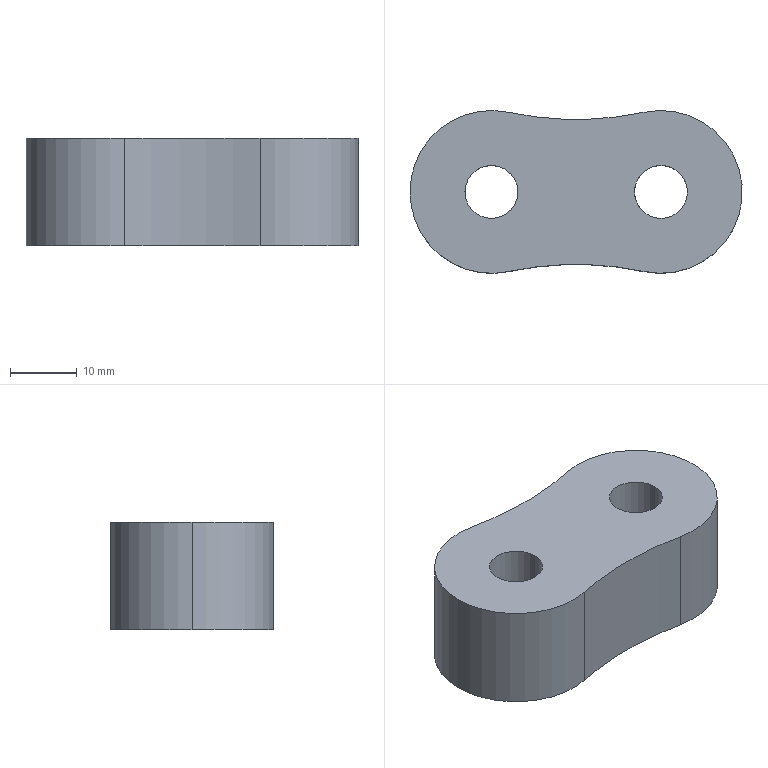Part | STEP file | Outer chain link pad block | 1 solid | 14 faces | box 49.79 x 24.39 x 16.175 mm | volume 15316 mm3 | cylinder 9 | plane 5 | commonest cylinder face diameters 7.94 x4 24.39 x3 97.627 x2
STEP:
#1=CARTESIAN_POINT('',(0.,0.,0.));
#2=DIRECTION('',(0.,0.,1.));
#3=DIRECTION('',(1.,0.,0.));
#4=AXIS2_PLACEMENT_3D('',#1,#2,#3);
#5=CARTESIAN_POINT('',(8.73,-0.05,-12.745));
#6=VERTEX_POINT('',#5);
#7=CARTESIAN_POINT('',(8.73,-0.05,-12.645));
#8=VERTEX_POINT('',#7);
#9=CARTESIAN_POINT('',(8.73,-0.05,0.));
#10=DIRECTION('',(0.,0.,1.));
#11=VECTOR('',#10,1.);
#12=LINE('',#9,#11);
#13=CARTESIAN_POINT('',(12.7,0.,0.));
#14=DIRECTION('',(0.,0.,1.));
#15=DIRECTION('',(1.,0.,0.));
#16=AXIS2_PLACEMENT_3D('',#13,#14,#15);
#17=CYLINDRICAL_SURFACE('',#16,3.97);
#18=CARTESIAN_POINT('',(3.154,0.));
#19=DIRECTION('',(0.,1.));
#20=VECTOR('',#19,1.);
#21=LINE('',#18,#20);
#22=(GEOMETRIC_REPRESENTATION_CONTEXT(2)PARAMETRIC_REPRESENTATION_CONTEXT()REPRESENTATION_CONTEXT('',''));
#23=DEFINITIONAL_REPRESENTATION('',(#21),#22);
#24=PCURVE('',#17,#23);
#25=CARTESIAN_POINT('',(15.,-0.05,-12.645));
#26=DIRECTION('',(0.,-1.,0.));
#27=DIRECTION('',(0.,0.,-1.));
#28=AXIS2_PLACEMENT_3D('',#25,#26,#27);
#29=PLANE('',#28);
#30=CARTESIAN_POINT('',(-12.645,-6.27));
#31=DIRECTION('',(-1.,0.));
#32=VECTOR('',#31,1.);
#33=LINE('',#30,#32);
#34=(GEOMETRIC_REPRESENTATION_CONTEXT(2)PARAMETRIC_REPRESENTATION_CONTEXT()REPRESENTATION_CONTEXT('',''));
#35=DEFINITIONAL_REPRESENTATION('',(#33),#34);
#36=PCURVE('',#29,#35);
#37=SURFACE_CURVE('',#12,(#24,#36),.PCURVE_S1.);
#38=EDGE_CURVE('',#6,#8,#37,.T.);
#39=ORIENTED_EDGE('',*,*,#38,.F.);
#40=CARTESIAN_POINT('',(16.67,0.,-12.745));
#41=VERTEX_POINT('',#40);
#42=CARTESIAN_POINT('',(12.7,0.,-12.745));
#43=DIRECTION('',(0.,0.,1.));
#44=DIRECTION('',(1.,0.,0.));
#45=AXIS2_PLACEMENT_3D('',#42,#43,#44);
#46=CIRCLE('',#45,3.97);
#47=CARTESIAN_POINT('',(0.,-12.745));
#48=DIRECTION('',(1.,0.));
#49=VECTOR('',#48,1.);
#50=LINE('',#47,#49);
#51=(GEOMETRIC_REPRESENTATION_CONTEXT(2)PARAMETRIC_REPRESENTATION_CONTEXT()REPRESENTATION_CONTEXT('',''));
#52=DEFINITIONAL_REPRESENTATION('',(#50),#51);
#53=PCURVE('',#17,#52);
#54=CARTESIAN_POINT('',(6.35,29.836,-12.745));
#55=DIRECTION('',(0.,0.,1.));
#56=DIRECTION('',(1.,0.,0.));
#57=AXIS2_PLACEMENT_3D('',#54,#55,#56);
#58=PLANE('',#57);
#59=CARTESIAN_POINT('',(6.35,-29.836));
#60=DIRECTION('',(1.,0.));
#61=AXIS2_PLACEMENT_2D('',#59,#60);
#62=CIRCLE('',#61,3.97);
#63=(GEOMETRIC_REPRESENTATION_CONTEXT(2)PARAMETRIC_REPRESENTATION_CONTEXT()REPRESENTATION_CONTEXT('',''));
#64=DEFINITIONAL_REPRESENTATION('',(#62),#63);
#65=PCURVE('',#58,#64);
#66=SURFACE_CURVE('',#46,(#53,#65),.PCURVE_S1.);
#67=EDGE_CURVE('',#6,#41,#66,.T.);
#68=ORIENTED_EDGE('',*,*,#67,.T.);
#69=CARTESIAN_POINT('',(16.67,0.,3.43));
#70=VERTEX_POINT('',#69);
#71=CARTESIAN_POINT('',(16.67,0.,0.));
#72=DIRECTION('',(0.,0.,1.));
#73=VECTOR('',#72,1.);
#74=LINE('',#71,#73);
#75=CARTESIAN_POINT('',(6.283,0.));
#76=DIRECTION('',(0.,1.));
#77=VECTOR('',#76,1.);
#78=LINE('',#75,#77);
#79=(GEOMETRIC_REPRESENTATION_CONTEXT(2)PARAMETRIC_REPRESENTATION_CONTEXT()REPRESENTATION_CONTEXT('',''));
#80=DEFINITIONAL_REPRESENTATION('',(#78),#79);
#81=PCURVE('',#17,#80);
#82=CARTESIAN_POINT('',(12.7,0.,0.));
#83=DIRECTION('',(0.,0.,1.));
#84=DIRECTION('',(1.,0.,0.));
#85=AXIS2_PLACEMENT_3D('',#82,#83,#84);
#86=CYLINDRICAL_SURFACE('',#85,3.97);
#87=CARTESIAN_POINT('',(0.,0.));
#88=DIRECTION('',(0.,1.));
#89=VECTOR('',#88,1.);
#90=LINE('',#87,#89);
#91=(GEOMETRIC_REPRESENTATION_CONTEXT(2)PARAMETRIC_REPRESENTATION_CONTEXT()REPRESENTATION_CONTEXT('',''));
#92=DEFINITIONAL_REPRESENTATION('',(#90),#91);
#93=PCURVE('',#86,#92);
#94=SURFACE_CURVE('',#74,(#81,#93),.PCURVE_S1.);
#95=EDGE_CURVE('',#41,#70,#94,.T.);
#96=ORIENTED_EDGE('',*,*,#95,.T.);
#97=CARTESIAN_POINT('',(8.73,0.,3.43));
#98=VERTEX_POINT('',#97);
#99=CARTESIAN_POINT('',(12.7,0.,3.43));
#100=DIRECTION('',(0.,0.,1.));
#101=DIRECTION('',(1.,0.,0.));
#102=AXIS2_PLACEMENT_3D('',#99,#100,#101);
#103=CIRCLE('',#102,3.97);
#104=CARTESIAN_POINT('',(0.,3.43));
#105=DIRECTION('',(1.,0.));
#106=VECTOR('',#105,1.);
#107=LINE('',#104,#106);
#108=(GEOMETRIC_REPRESENTATION_CONTEXT(2)PARAMETRIC_REPRESENTATION_CONTEXT()REPRESENTATION_CONTEXT('',''));
#109=DEFINITIONAL_REPRESENTATION('',(#107),#108);
#110=PCURVE('',#17,#109);
#111=CARTESIAN_POINT('',(-6.35,-29.836,3.43));
#112=DIRECTION('',(0.,0.,1.));
#113=DIRECTION('',(1.,0.,0.));
#114=AXIS2_PLACEMENT_3D('',#111,#112,#113);
#115=PLANE('',#114);
#116=CARTESIAN_POINT('',(19.05,29.836));
#117=DIRECTION('',(1.,0.));
#118=AXIS2_PLACEMENT_2D('',#116,#117);
#119=CIRCLE('',#118,3.97);
#120=(GEOMETRIC_REPRESENTATION_CONTEXT(2)PARAMETRIC_REPRESENTATION_CONTEXT()REPRESENTATION_CONTEXT('',''));
#121=DEFINITIONAL_REPRESENTATION('',(#119),#120);
#122=PCURVE('',#115,#121);
#123=SURFACE_CURVE('',#103,(#110,#122),.PCURVE_S1.);
#124=EDGE_CURVE('',#98,#70,#123,.T.);
#125=ORIENTED_EDGE('',*,*,#124,.F.);
#126=CARTESIAN_POINT('',(8.73,0.,-12.645));
#127=VERTEX_POINT('',#126);
#128=CARTESIAN_POINT('',(8.73,0.,0.));
#129=DIRECTION('',(0.,0.,1.));
#130=VECTOR('',#129,1.);
#131=LINE('',#128,#130);
#132=CARTESIAN_POINT('',(3.142,0.));
#133=DIRECTION('',(0.,1.));
#134=VECTOR('',#133,1.);
#135=LINE('',#132,#134);
#136=(GEOMETRIC_REPRESENTATION_CONTEXT(2)PARAMETRIC_REPRESENTATION_CONTEXT()REPRESENTATION_CONTEXT('',''));
#137=DEFINITIONAL_REPRESENTATION('',(#135),#136);
#138=PCURVE('',#17,#137);
#139=CARTESIAN_POINT('',(3.142,0.));
#140=DIRECTION('',(0.,1.));
#141=VECTOR('',#140,1.);
#142=LINE('',#139,#141);
#143=(GEOMETRIC_REPRESENTATION_CONTEXT(2)PARAMETRIC_REPRESENTATION_CONTEXT()REPRESENTATION_CONTEXT('',''));
#144=DEFINITIONAL_REPRESENTATION('',(#142),#143);
#145=PCURVE('',#86,#144);
#146=SURFACE_CURVE('',#131,(#138,#145),.PCURVE_S1.);
#147=EDGE_CURVE('',#127,#98,#146,.T.);
#148=ORIENTED_EDGE('',*,*,#147,.F.);
#149=CARTESIAN_POINT('',(12.7,0.,-12.645));
#150=DIRECTION('',(0.,0.,1.));
#151=DIRECTION('',(-1.,0.,0.));
#152=AXIS2_PLACEMENT_3D('',#149,#150,#151);
#153=CIRCLE('',#152,3.97);
#154=CARTESIAN_POINT('',(3.142,-12.645));
#155=DIRECTION('',(1.,0.));
#156=VECTOR('',#155,1.);
#157=LINE('',#154,#156);
#158=(GEOMETRIC_REPRESENTATION_CONTEXT(2)PARAMETRIC_REPRESENTATION_CONTEXT()REPRESENTATION_CONTEXT('',''));
#159=DEFINITIONAL_REPRESENTATION('',(#157),#158);
#160=PCURVE('',#17,#159);
#161=CARTESIAN_POINT('',(0.,0.,-12.645));
#162=DIRECTION('',(0.,0.,-1.));
#163=DIRECTION('',(-1.,0.,0.));
#164=AXIS2_PLACEMENT_3D('',#161,#162,#163);
#165=PLANE('',#164);
#166=CARTESIAN_POINT('',(-8.73,0.));
#167=CARTESIAN_POINT('',(-8.73,-6.876));
#168=CARTESIAN_POINT('',(-14.685,-3.438));
#169=CARTESIAN_POINT('',(-20.64,0.));
#170=CARTESIAN_POINT('',(-14.685,3.438));
#171=CARTESIAN_POINT('',(-8.73,6.876));
#172=CARTESIAN_POINT('',(-8.73,0.));
#173=(BOUNDED_CURVE()B_SPLINE_CURVE(2,(#166,#167,#168,#169,#170,#171,#172),.UNSPECIFIED.,.T.,.F.)B_SPLINE_CURVE_WITH_KNOTS((1,2,2,2,2,1),(-2.094,0.,2.094,4.189,6.283,8.378),.UNSPECIFIED.)CURVE()GEOMETRIC_REPRESENTATION_ITEM()RATIONAL_B_SPLINE_CURVE((1.,0.5,1.,0.5,1.,0.5,1.))REPRESENTATION_ITEM(''));
#174=(GEOMETRIC_REPRESENTATION_CONTEXT(2)PARAMETRIC_REPRESENTATION_CONTEXT()REPRESENTATION_CONTEXT('',''));
#175=DEFINITIONAL_REPRESENTATION('',(#173),#174);
#176=PCURVE('',#165,#175);
#177=SURFACE_CURVE('',#153,(#160,#176),.PCURVE_S1.);
#178=EDGE_CURVE('',#127,#8,#177,.T.);
#179=ORIENTED_EDGE('',*,*,#178,.T.);
#180=EDGE_LOOP('',(#39,#68,#96,#125,#148,#179));
#181=FACE_BOUND('',#180,.F.);
#182=ADVANCED_FACE('',(#181),#17,.F.);
#183=CARTESIAN_POINT('',(-8.73,-0.05,-12.645));
#184=VERTEX_POINT('',#183);
#185=CARTESIAN_POINT('',(-8.73,-0.05,-12.745));
#186=VERTEX_POINT('',#185);
#187=CARTESIAN_POINT('',(-8.73,-0.05,0.));
#188=DIRECTION('',(0.,0.,-1.));
#189=VECTOR('',#188,1.);
#190=LINE('',#187,#189);
#191=CARTESIAN_POINT('',(-12.7,0.,0.));
#192=DIRECTION('',(0.,0.,1.));
#193=DIRECTION('',(1.,0.,0.));
#194=AXIS2_PLACEMENT_3D('',#191,#192,#193);
#195=CYLINDRICAL_SURFACE('',#194,3.97);
#196=CARTESIAN_POINT('',(6.271,0.));
#197=DIRECTION('',(0.,-1.));
#198=VECTOR('',#197,1.);
#199=LINE('',#196,#198);
#200=(GEOMETRIC_REPRESENTATION_CONTEXT(2)PARAMETRIC_REPRESENTATION_CONTEXT()REPRESENTATION_CONTEXT('',''));
#201=DEFINITIONAL_REPRESENTATION('',(#199),#200);
#202=PCURVE('',#195,#201);
#203=CARTESIAN_POINT('',(-12.645,-23.73));
#204=DIRECTION('',(1.,0.));
#205=VECTOR('',#204,1.);
#206=LINE('',#203,#205);
#207=(GEOMETRIC_REPRESENTATION_CONTEXT(2)PARAMETRIC_REPRESENTATION_CONTEXT()REPRESENTATION_CONTEXT('',''));
#208=DEFINITIONAL_REPRESENTATION('',(#206),#207);
#209=PCURVE('',#29,#208);
#210=SURFACE_CURVE('',#190,(#202,#209),.PCURVE_S1.);
#211=EDGE_CURVE('',#184,#186,#210,.T.);
#212=ORIENTED_EDGE('',*,*,#211,.F.);
#213=CARTESIAN_POINT('',(-8.73,0.,-12.645));
#214=VERTEX_POINT('',#213);
#215=CARTESIAN_POINT('',(-12.7,0.,-12.645));
#216=DIRECTION('',(0.,0.,1.));
#217=DIRECTION('',(-1.,0.,0.));
#218=AXIS2_PLACEMENT_3D('',#215,#216,#217);
#219=CIRCLE('',#218,3.97);
#220=CARTESIAN_POINT('',(3.142,-12.645));
#221=DIRECTION('',(1.,0.));
#222=VECTOR('',#221,1.);
#223=LINE('',#220,#222);
#224=(GEOMETRIC_REPRESENTATION_CONTEXT(2)PARAMETRIC_REPRESENTATION_CONTEXT()REPRESENTATION_CONTEXT('',''));
#225=DEFINITIONAL_REPRESENTATION('',(#223),#224);
#226=PCURVE('',#195,#225);
#227=CARTESIAN_POINT('',(16.67,0.));
#228=CARTESIAN_POINT('',(16.67,-6.876));
#229=CARTESIAN_POINT('',(10.715,-3.438));
#230=CARTESIAN_POINT('',(4.76,0.));
#231=CARTESIAN_POINT('',(10.715,3.438));
#232=CARTESIAN_POINT('',(16.67,6.876));
#233=CARTESIAN_POINT('',(16.67,0.));
#234=(BOUNDED_CURVE()B_SPLINE_CURVE(2,(#227,#228,#229,#230,#231,#232,#233),.UNSPECIFIED.,.T.,.F.)B_SPLINE_CURVE_WITH_KNOTS((1,2,2,2,2,1),(-2.094,0.,2.094,4.189,6.283,8.378),.UNSPECIFIED.)CURVE()GEOMETRIC_REPRESENTATION_ITEM()RATIONAL_B_SPLINE_CURVE((1.,0.5,1.,0.5,1.,0.5,1.))REPRESENTATION_ITEM(''));
#235=(GEOMETRIC_REPRESENTATION_CONTEXT(2)PARAMETRIC_REPRESENTATION_CONTEXT()REPRESENTATION_CONTEXT('',''));
#236=DEFINITIONAL_REPRESENTATION('',(#234),#235);
#237=PCURVE('',#165,#236);
#238=SURFACE_CURVE('',#219,(#226,#237),.PCURVE_S1.);
#239=EDGE_CURVE('',#184,#214,#238,.T.);
#240=ORIENTED_EDGE('',*,*,#239,.T.);
#241=CARTESIAN_POINT('',(-8.73,0.,3.43));
#242=VERTEX_POINT('',#241);
#243=CARTESIAN_POINT('',(-8.73,0.,0.));
#244=DIRECTION('',(0.,0.,1.));
#245=VECTOR('',#244,1.);
#246=LINE('',#243,#245);
#247=CARTESIAN_POINT('',(6.283,0.));
#248=DIRECTION('',(0.,1.));
#249=VECTOR('',#248,1.);
#250=LINE('',#247,#249);
#251=(GEOMETRIC_REPRESENTATION_CONTEXT(2)PARAMETRIC_REPRESENTATION_CONTEXT()REPRESENTATION_CONTEXT('',''));
#252=DEFINITIONAL_REPRESENTATION('',(#250),#251);
#253=PCURVE('',#195,#252);
#254=CARTESIAN_POINT('',(-12.7,0.,0.));
#255=DIRECTION('',(0.,0.,1.));
#256=DIRECTION('',(1.,0.,0.));
#257=AXIS2_PLACEMENT_3D('',#254,#255,#256);
#258=CYLINDRICAL_SURFACE('',#257,3.97);
#259=CARTESIAN_POINT('',(0.,0.));
#260=DIRECTION('',(0.,1.));
#261=VECTOR('',#260,1.);
#262=LINE('',#259,#261);
#263=(GEOMETRIC_REPRESENTATION_CONTEXT(2)PARAMETRIC_REPRESENTATION_CONTEXT()REPRESENTATION_CONTEXT('',''));
#264=DEFINITIONAL_REPRESENTATION('',(#262),#263);
#265=PCURVE('',#258,#264);
#266=SURFACE_CURVE('',#246,(#253,#265),.PCURVE_S1.);
#267=EDGE_CURVE('',#214,#242,#266,.T.);
#268=ORIENTED_EDGE('',*,*,#267,.T.);
#269=CARTESIAN_POINT('',(-16.67,0.,3.43));
#270=VERTEX_POINT('',#269);
#271=CARTESIAN_POINT('',(-12.7,0.,3.43));
#272=DIRECTION('',(0.,0.,1.));
#273=DIRECTION('',(1.,0.,0.));
#274=AXIS2_PLACEMENT_3D('',#271,#272,#273);
#275=CIRCLE('',#274,3.97);
#276=CARTESIAN_POINT('',(0.,3.43));
#277=DIRECTION('',(1.,0.));
#278=VECTOR('',#277,1.);
#279=LINE('',#276,#278);
#280=(GEOMETRIC_REPRESENTATION_CONTEXT(2)PARAMETRIC_REPRESENTATION_CONTEXT()REPRESENTATION_CONTEXT('',''));
#281=DEFINITIONAL_REPRESENTATION('',(#279),#280);
#282=PCURVE('',#195,#281);
#283=CARTESIAN_POINT('',(-6.35,29.836));
#284=DIRECTION('',(1.,0.));
#285=AXIS2_PLACEMENT_2D('',#283,#284);
#286=CIRCLE('',#285,3.97);
#287=(GEOMETRIC_REPRESENTATION_CONTEXT(2)PARAMETRIC_REPRESENTATION_CONTEXT()REPRESENTATION_CONTEXT('',''));
#288=DEFINITIONAL_REPRESENTATION('',(#286),#287);
#289=PCURVE('',#115,#288);
#290=SURFACE_CURVE('',#275,(#282,#289),.PCURVE_S1.);
#291=EDGE_CURVE('',#270,#242,#290,.T.);
#292=ORIENTED_EDGE('',*,*,#291,.F.);
#293=CARTESIAN_POINT('',(-16.67,0.,-12.745));
#294=VERTEX_POINT('',#293);
#295=CARTESIAN_POINT('',(-16.67,0.,0.));
#296=DIRECTION('',(0.,0.,1.));
#297=VECTOR('',#296,1.);
#298=LINE('',#295,#297);
#299=CARTESIAN_POINT('',(3.142,0.));
#300=DIRECTION('',(0.,1.));
#301=VECTOR('',#300,1.);
#302=LINE('',#299,#301);
#303=(GEOMETRIC_REPRESENTATION_CONTEXT(2)PARAMETRIC_REPRESENTATION_CONTEXT()REPRESENTATION_CONTEXT('',''));
#304=DEFINITIONAL_REPRESENTATION('',(#302),#303);
#305=PCURVE('',#195,#304);
#306=CARTESIAN_POINT('',(3.142,0.));
#307=DIRECTION('',(0.,1.));
#308=VECTOR('',#307,1.);
#309=LINE('',#306,#308);
#310=(GEOMETRIC_REPRESENTATION_CONTEXT(2)PARAMETRIC_REPRESENTATION_CONTEXT()REPRESENTATION_CONTEXT('',''));
#311=DEFINITIONAL_REPRESENTATION('',(#309),#310);
#312=PCURVE('',#258,#311);
#313=SURFACE_CURVE('',#298,(#305,#312),.PCURVE_S1.);
#314=EDGE_CURVE('',#294,#270,#313,.T.);
#315=ORIENTED_EDGE('',*,*,#314,.F.);
#316=CARTESIAN_POINT('',(-12.7,0.,-12.745));
#317=DIRECTION('',(0.,0.,1.));
#318=DIRECTION('',(1.,0.,0.));
#319=AXIS2_PLACEMENT_3D('',#316,#317,#318);
#320=CIRCLE('',#319,3.97);
#321=CARTESIAN_POINT('',(0.,-12.745));
#322=DIRECTION('',(1.,0.));
#323=VECTOR('',#322,1.);
#324=LINE('',#321,#323);
#325=(GEOMETRIC_REPRESENTATION_CONTEXT(2)PARAMETRIC_REPRESENTATION_CONTEXT()REPRESENTATION_CONTEXT('',''));
#326=DEFINITIONAL_REPRESENTATION('',(#324),#325);
#327=PCURVE('',#195,#326);
#328=CARTESIAN_POINT('',(-19.05,-29.836));
#329=DIRECTION('',(1.,0.));
#330=AXIS2_PLACEMENT_2D('',#328,#329);
#331=CIRCLE('',#330,3.97);
#332=(GEOMETRIC_REPRESENTATION_CONTEXT(2)PARAMETRIC_REPRESENTATION_CONTEXT()REPRESENTATION_CONTEXT('',''));
#333=DEFINITIONAL_REPRESENTATION('',(#331),#332);
#334=PCURVE('',#58,#333);
#335=SURFACE_CURVE('',#320,(#327,#334),.PCURVE_S1.);
#336=EDGE_CURVE('',#294,#186,#335,.T.);
#337=ORIENTED_EDGE('',*,*,#336,.T.);
#338=EDGE_LOOP('',(#212,#240,#268,#292,#315,#337));
#339=FACE_BOUND('',#338,.F.);
#340=ADVANCED_FACE('',(#339),#195,.F.);
#341=CARTESIAN_POINT('',(-24.895,0.,3.43));
#342=VERTEX_POINT('',#341);
#343=CARTESIAN_POINT('',(-10.161,-11.928,3.43));
#344=VERTEX_POINT('',#343);
#345=CARTESIAN_POINT('',(-12.7,0.,3.43));
#346=DIRECTION('',(0.,0.,1.));
#347=DIRECTION('',(1.,0.,0.));
#348=AXIS2_PLACEMENT_3D('',#345,#346,#347);
#349=CIRCLE('',#348,12.195);
#350=CARTESIAN_POINT('',(-12.7,0.,3.43));
#351=DIRECTION('',(0.,0.,-1.));
#352=DIRECTION('',(-1.,0.,0.));
#353=AXIS2_PLACEMENT_3D('',#350,#351,#352);
#354=CYLINDRICAL_SURFACE('',#353,12.195);
#355=CARTESIAN_POINT('',(9.425,0.));
#356=DIRECTION('',(-1.,0.));
#357=VECTOR('',#356,1.);
#358=LINE('',#355,#357);
#359=(GEOMETRIC_REPRESENTATION_CONTEXT(2)PARAMETRIC_REPRESENTATION_CONTEXT()REPRESENTATION_CONTEXT('',''));
#360=DEFINITIONAL_REPRESENTATION('',(#358),#359);
#361=PCURVE('',#354,#360);
#362=CARTESIAN_POINT('',(-6.35,29.836));
#363=DIRECTION('',(1.,0.));
#364=AXIS2_PLACEMENT_2D('',#362,#363);
#365=CIRCLE('',#364,12.195);
#366=(GEOMETRIC_REPRESENTATION_CONTEXT(2)PARAMETRIC_REPRESENTATION_CONTEXT()REPRESENTATION_CONTEXT('',''));
#367=DEFINITIONAL_REPRESENTATION('',(#365),#366);
#368=PCURVE('',#115,#367);
#369=SURFACE_CURVE('',#349,(#361,#368),.PCURVE_S1.);
#370=EDGE_CURVE('',#342,#344,#369,.T.);
#371=ORIENTED_EDGE('',*,*,#370,.F.);
#372=CARTESIAN_POINT('',(-24.895,0.,-12.745));
#373=VERTEX_POINT('',#372);
#374=CARTESIAN_POINT('',(-24.895,0.,3.43));
#375=DIRECTION('',(0.,0.,-1.));
#376=VECTOR('',#375,1.);
#377=LINE('',#374,#376);
#378=CARTESIAN_POINT('',(6.283,0.));
#379=DIRECTION('',(0.,1.));
#380=VECTOR('',#379,1.);
#381=LINE('',#378,#380);
#382=(GEOMETRIC_REPRESENTATION_CONTEXT(2)PARAMETRIC_REPRESENTATION_CONTEXT()REPRESENTATION_CONTEXT('',''));
#383=DEFINITIONAL_REPRESENTATION('',(#381),#382);
#384=PCURVE('',#354,#383);
#385=CARTESIAN_POINT('',(-12.7,0.,3.43));
#386=DIRECTION('',(0.,0.,-1.));
#387=DIRECTION('',(-1.,0.,0.));
#388=AXIS2_PLACEMENT_3D('',#385,#386,#387);
#389=CYLINDRICAL_SURFACE('',#388,12.195);
#390=CARTESIAN_POINT('',(0.,0.));
#391=DIRECTION('',(0.,1.));
#392=VECTOR('',#391,1.);
#393=LINE('',#390,#392);
#394=(GEOMETRIC_REPRESENTATION_CONTEXT(2)PARAMETRIC_REPRESENTATION_CONTEXT()REPRESENTATION_CONTEXT('',''));
#395=DEFINITIONAL_REPRESENTATION('',(#393),#394);
#396=PCURVE('',#389,#395);
#397=SURFACE_CURVE('',#377,(#384,#396),.PCURVE_S1.);
#398=EDGE_CURVE('',#342,#373,#397,.T.);
#399=ORIENTED_EDGE('',*,*,#398,.T.);
#400=CARTESIAN_POINT('',(-10.161,-11.928,-12.745));
#401=VERTEX_POINT('',#400);
#402=CARTESIAN_POINT('',(-12.7,0.,-12.745));
#403=DIRECTION('',(0.,0.,1.));
#404=DIRECTION('',(1.,0.,0.));
#405=AXIS2_PLACEMENT_3D('',#402,#403,#404);
#406=CIRCLE('',#405,12.195);
#407=CARTESIAN_POINT('',(9.425,16.175));
#408=DIRECTION('',(-1.,0.));
#409=VECTOR('',#408,1.);
#410=LINE('',#407,#409);
#411=(GEOMETRIC_REPRESENTATION_CONTEXT(2)PARAMETRIC_REPRESENTATION_CONTEXT()REPRESENTATION_CONTEXT('',''));
#412=DEFINITIONAL_REPRESENTATION('',(#410),#411);
#413=PCURVE('',#354,#412);
#414=CARTESIAN_POINT('',(-19.05,-29.836));
#415=DIRECTION('',(1.,0.));
#416=AXIS2_PLACEMENT_2D('',#414,#415);
#417=CIRCLE('',#416,12.195);
#418=(GEOMETRIC_REPRESENTATION_CONTEXT(2)PARAMETRIC_REPRESENTATION_CONTEXT()REPRESENTATION_CONTEXT('',''));
#419=DEFINITIONAL_REPRESENTATION('',(#417),#418);
#420=PCURVE('',#58,#419);
#421=SURFACE_CURVE('',#406,(#413,#420),.PCURVE_S1.);
#422=EDGE_CURVE('',#373,#401,#421,.T.);
#423=ORIENTED_EDGE('',*,*,#422,.T.);
#424=CARTESIAN_POINT('',(-10.161,-11.928,3.43));
#425=DIRECTION('',(0.,0.,-1.));
#426=VECTOR('',#425,1.);
#427=LINE('',#424,#426);
#428=CARTESIAN_POINT('',(4.503,0.));
#429=DIRECTION('',(0.,1.));
#430=VECTOR('',#429,1.);
#431=LINE('',#428,#430);
#432=(GEOMETRIC_REPRESENTATION_CONTEXT(2)PARAMETRIC_REPRESENTATION_CONTEXT()REPRESENTATION_CONTEXT('',''));
#433=DEFINITIONAL_REPRESENTATION('',(#431),#432);
#434=PCURVE('',#354,#433);
#435=CARTESIAN_POINT('',(0.,-59.672,3.43));
#436=DIRECTION('',(0.,0.,-1.));
#437=DIRECTION('',(-1.,0.,0.));
#438=AXIS2_PLACEMENT_3D('',#435,#436,#437);
#439=CYLINDRICAL_SURFACE('',#438,48.814);
#440=CARTESIAN_POINT('',(1.361,0.));
#441=DIRECTION('',(0.,1.));
#442=VECTOR('',#441,1.);
#443=LINE('',#440,#442);
#444=(GEOMETRIC_REPRESENTATION_CONTEXT(2)PARAMETRIC_REPRESENTATION_CONTEXT()REPRESENTATION_CONTEXT('',''));
#445=DEFINITIONAL_REPRESENTATION('',(#443),#444);
#446=PCURVE('',#439,#445);
#447=SURFACE_CURVE('',#427,(#434,#446),.PCURVE_S1.);
#448=EDGE_CURVE('',#344,#401,#447,.T.);
#449=ORIENTED_EDGE('',*,*,#448,.F.);
#450=EDGE_LOOP('',(#371,#399,#423,#449));
#451=FACE_BOUND('',#450,.T.);
#452=ADVANCED_FACE('',(#451),#354,.T.);
#453=CARTESIAN_POINT('',(10.161,-11.928,3.43));
#454=VERTEX_POINT('',#453);
#455=CARTESIAN_POINT('',(0.,-59.672,3.43));
#456=DIRECTION('',(0.,0.,-1.));
#457=DIRECTION('',(1.,0.,0.));
#458=AXIS2_PLACEMENT_3D('',#455,#456,#457);
#459=CIRCLE('',#458,48.814);
#460=CARTESIAN_POINT('',(-3.142,0.));
#461=DIRECTION('',(1.,0.));
#462=VECTOR('',#461,1.);
#463=LINE('',#460,#462);
#464=(GEOMETRIC_REPRESENTATION_CONTEXT(2)PARAMETRIC_REPRESENTATION_CONTEXT()REPRESENTATION_CONTEXT('',''));
#465=DEFINITIONAL_REPRESENTATION('',(#463),#464);
#466=PCURVE('',#439,#465);
#467=CARTESIAN_POINT('',(55.164,-29.836));
#468=CARTESIAN_POINT('',(55.164,-114.384));
#469=CARTESIAN_POINT('',(-18.057,-72.11));
#470=CARTESIAN_POINT('',(-91.277,-29.836));
#471=CARTESIAN_POINT('',(-18.057,12.438));
#472=CARTESIAN_POINT('',(55.164,54.712));
#473=CARTESIAN_POINT('',(55.164,-29.836));
#474=(BOUNDED_CURVE()B_SPLINE_CURVE(2,(#467,#468,#469,#470,#471,#472,#473),.UNSPECIFIED.,.T.,.F.)B_SPLINE_CURVE_WITH_KNOTS((1,2,2,2,2,1),(-2.094,0.,2.094,4.189,6.283,8.378),.UNSPECIFIED.)CURVE()GEOMETRIC_REPRESENTATION_ITEM()RATIONAL_B_SPLINE_CURVE((1.,0.5,1.,0.5,1.,0.5,1.))REPRESENTATION_ITEM(''));
#475=(GEOMETRIC_REPRESENTATION_CONTEXT(2)PARAMETRIC_REPRESENTATION_CONTEXT()REPRESENTATION_CONTEXT('',''));
#476=DEFINITIONAL_REPRESENTATION('',(#474),#475);
#477=PCURVE('',#115,#476);
#478=SURFACE_CURVE('',#459,(#466,#477),.PCURVE_S1.);
#479=EDGE_CURVE('',#344,#454,#478,.T.);
#480=ORIENTED_EDGE('',*,*,#479,.T.);
#481=CARTESIAN_POINT('',(10.161,-11.928,-12.745));
#482=VERTEX_POINT('',#481);
#483=CARTESIAN_POINT('',(10.161,-11.928,3.43));
#484=DIRECTION('',(0.,0.,-1.));
#485=VECTOR('',#484,1.);
#486=LINE('',#483,#485);
#487=CARTESIAN_POINT('',(1.78,0.));
#488=DIRECTION('',(0.,1.));
#489=VECTOR('',#488,1.);
#490=LINE('',#487,#489);
#491=(GEOMETRIC_REPRESENTATION_CONTEXT(2)PARAMETRIC_REPRESENTATION_CONTEXT()REPRESENTATION_CONTEXT('',''));
#492=DEFINITIONAL_REPRESENTATION('',(#490),#491);
#493=PCURVE('',#439,#492);
#494=CARTESIAN_POINT('',(12.7,0.,3.43));
#495=DIRECTION('',(0.,0.,-1.));
#496=DIRECTION('',(-1.,0.,0.));
#497=AXIS2_PLACEMENT_3D('',#494,#495,#496);
#498=CYLINDRICAL_SURFACE('',#497,12.195);
#499=CARTESIAN_POINT('',(4.922,0.));
#500=DIRECTION('',(0.,1.));
#501=VECTOR('',#500,1.);
#502=LINE('',#499,#501);
#503=(GEOMETRIC_REPRESENTATION_CONTEXT(2)PARAMETRIC_REPRESENTATION_CONTEXT()REPRESENTATION_CONTEXT('',''));
#504=DEFINITIONAL_REPRESENTATION('',(#502),#503);
#505=PCURVE('',#498,#504);
#506=SURFACE_CURVE('',#486,(#493,#505),.PCURVE_S1.);
#507=EDGE_CURVE('',#454,#482,#506,.T.);
#508=ORIENTED_EDGE('',*,*,#507,.T.);
#509=CARTESIAN_POINT('',(0.,-59.672,-12.745));
#510=DIRECTION('',(0.,0.,-1.));
#511=DIRECTION('',(1.,0.,0.));
#512=AXIS2_PLACEMENT_3D('',#509,#510,#511);
#513=CIRCLE('',#512,48.814);
#514=CARTESIAN_POINT('',(-3.142,16.175));
#515=DIRECTION('',(1.,0.));
#516=VECTOR('',#515,1.);
#517=LINE('',#514,#516);
#518=(GEOMETRIC_REPRESENTATION_CONTEXT(2)PARAMETRIC_REPRESENTATION_CONTEXT()REPRESENTATION_CONTEXT('',''));
#519=DEFINITIONAL_REPRESENTATION('',(#517),#518);
#520=PCURVE('',#439,#519);
#521=CARTESIAN_POINT('',(42.464,-89.508));
#522=CARTESIAN_POINT('',(42.464,-174.056));
#523=CARTESIAN_POINT('',(-30.757,-131.782));
#524=CARTESIAN_POINT('',(-103.977,-89.508));
#525=CARTESIAN_POINT('',(-30.757,-47.234));
#526=CARTESIAN_POINT('',(42.464,-4.96));
#527=CARTESIAN_POINT('',(42.464,-89.508));
#528=(BOUNDED_CURVE()B_SPLINE_CURVE(2,(#521,#522,#523,#524,#525,#526,#527),.UNSPECIFIED.,.T.,.F.)B_SPLINE_CURVE_WITH_KNOTS((1,2,2,2,2,1),(-2.094,0.,2.094,4.189,6.283,8.378),.UNSPECIFIED.)CURVE()GEOMETRIC_REPRESENTATION_ITEM()RATIONAL_B_SPLINE_CURVE((1.,0.5,1.,0.5,1.,0.5,1.))REPRESENTATION_ITEM(''));
#529=(GEOMETRIC_REPRESENTATION_CONTEXT(2)PARAMETRIC_REPRESENTATION_CONTEXT()REPRESENTATION_CONTEXT('',''));
#530=DEFINITIONAL_REPRESENTATION('',(#528),#529);
#531=PCURVE('',#58,#530);
#532=SURFACE_CURVE('',#513,(#520,#531),.PCURVE_S1.);
#533=EDGE_CURVE('',#401,#482,#532,.T.);
#534=ORIENTED_EDGE('',*,*,#533,.F.);
#535=ORIENTED_EDGE('',*,*,#448,.F.);
#536=EDGE_LOOP('',(#480,#508,#534,#535));
#537=FACE_BOUND('',#536,.F.);
#538=ADVANCED_FACE('',(#537),#439,.F.);
#539=ORIENTED_EDGE('',*,*,#507,.T.);
#540=CARTESIAN_POINT('',(10.161,11.928,-12.745));
#541=VERTEX_POINT('',#540);
#542=CARTESIAN_POINT('',(12.7,0.,-12.745));
#543=DIRECTION('',(0.,0.,1.));
#544=DIRECTION('',(1.,0.,0.));
#545=AXIS2_PLACEMENT_3D('',#542,#543,#544);
#546=CIRCLE('',#545,12.195);
#547=CARTESIAN_POINT('',(9.425,16.175));
#548=DIRECTION('',(-1.,0.));
#549=VECTOR('',#548,1.);
#550=LINE('',#547,#549);
#551=(GEOMETRIC_REPRESENTATION_CONTEXT(2)PARAMETRIC_REPRESENTATION_CONTEXT()REPRESENTATION_CONTEXT('',''));
#552=DEFINITIONAL_REPRESENTATION('',(#550),#551);
#553=PCURVE('',#498,#552);
#554=CARTESIAN_POINT('',(6.35,-29.836));
#555=DIRECTION('',(1.,0.));
#556=AXIS2_PLACEMENT_2D('',#554,#555);
#557=CIRCLE('',#556,12.195);
#558=(GEOMETRIC_REPRESENTATION_CONTEXT(2)PARAMETRIC_REPRESENTATION_CONTEXT()REPRESENTATION_CONTEXT('',''));
#559=DEFINITIONAL_REPRESENTATION('',(#557),#558);
#560=PCURVE('',#58,#559);
#561=SURFACE_CURVE('',#546,(#553,#560),.PCURVE_S1.);
#562=EDGE_CURVE('',#482,#541,#561,.T.);
#563=ORIENTED_EDGE('',*,*,#562,.T.);
#564=CARTESIAN_POINT('',(10.161,11.928,3.43));
#565=VERTEX_POINT('',#564);
#566=CARTESIAN_POINT('',(10.161,11.928,3.43));
#567=DIRECTION('',(0.,0.,-1.));
#568=VECTOR('',#567,1.);
#569=LINE('',#566,#568);
#570=CARTESIAN_POINT('',(1.361,0.));
#571=DIRECTION('',(0.,1.));
#572=VECTOR('',#571,1.);
#573=LINE('',#570,#572);
#574=(GEOMETRIC_REPRESENTATION_CONTEXT(2)PARAMETRIC_REPRESENTATION_CONTEXT()REPRESENTATION_CONTEXT('',''));
#575=DEFINITIONAL_REPRESENTATION('',(#573),#574);
#576=PCURVE('',#498,#575);
#577=CARTESIAN_POINT('',(0.,59.672,3.43));
#578=DIRECTION('',(0.,0.,-1.));
#579=DIRECTION('',(-1.,0.,0.));
#580=AXIS2_PLACEMENT_3D('',#577,#578,#579);
#581=CYLINDRICAL_SURFACE('',#580,48.814);
#582=CARTESIAN_POINT('',(4.503,0.));
#583=DIRECTION('',(0.,1.));
#584=VECTOR('',#583,1.);
#585=LINE('',#582,#584);
#586=(GEOMETRIC_REPRESENTATION_CONTEXT(2)PARAMETRIC_REPRESENTATION_CONTEXT()REPRESENTATION_CONTEXT('',''));
#587=DEFINITIONAL_REPRESENTATION('',(#585),#586);
#588=PCURVE('',#581,#587);
#589=SURFACE_CURVE('',#569,(#576,#588),.PCURVE_S1.);
#590=EDGE_CURVE('',#565,#541,#589,.T.);
#591=ORIENTED_EDGE('',*,*,#590,.F.);
#592=CARTESIAN_POINT('',(12.7,0.,3.43));
#593=DIRECTION('',(0.,0.,1.));
#594=DIRECTION('',(1.,0.,0.));
#595=AXIS2_PLACEMENT_3D('',#592,#593,#594);
#596=CIRCLE('',#595,12.195);
#597=CARTESIAN_POINT('',(9.425,0.));
#598=DIRECTION('',(-1.,0.));
#599=VECTOR('',#598,1.);
#600=LINE('',#597,#599);
#601=(GEOMETRIC_REPRESENTATION_CONTEXT(2)PARAMETRIC_REPRESENTATION_CONTEXT()REPRESENTATION_CONTEXT('',''));
#602=DEFINITIONAL_REPRESENTATION('',(#600),#601);
#603=PCURVE('',#498,#602);
#604=CARTESIAN_POINT('',(19.05,29.836));
#605=DIRECTION('',(1.,0.));
#606=AXIS2_PLACEMENT_2D('',#604,#605);
#607=CIRCLE('',#606,12.195);
#608=(GEOMETRIC_REPRESENTATION_CONTEXT(2)PARAMETRIC_REPRESENTATION_CONTEXT()REPRESENTATION_CONTEXT('',''));
#609=DEFINITIONAL_REPRESENTATION('',(#607),#608);
#610=PCURVE('',#115,#609);
#611=SURFACE_CURVE('',#596,(#603,#610),.PCURVE_S1.);
#612=EDGE_CURVE('',#454,#565,#611,.T.);
#613=ORIENTED_EDGE('',*,*,#612,.F.);
#614=EDGE_LOOP('',(#539,#563,#591,#613));
#615=FACE_BOUND('',#614,.T.);
#616=ADVANCED_FACE('',(#615),#498,.T.);
#617=CARTESIAN_POINT('',(-10.161,11.928,3.43));
#618=VERTEX_POINT('',#617);
#619=CARTESIAN_POINT('',(0.,59.672,3.43));
#620=DIRECTION('',(0.,0.,-1.));
#621=DIRECTION('',(1.,0.,0.));
#622=AXIS2_PLACEMENT_3D('',#619,#620,#621);
#623=CIRCLE('',#622,48.814);
#624=CARTESIAN_POINT('',(3.142,0.));
#625=DIRECTION('',(1.,0.));
#626=VECTOR('',#625,1.);
#627=LINE('',#624,#626);
#628=(GEOMETRIC_REPRESENTATION_CONTEXT(2)PARAMETRIC_REPRESENTATION_CONTEXT()REPRESENTATION_CONTEXT('',''));
#629=DEFINITIONAL_REPRESENTATION('',(#627),#628);
#630=PCURVE('',#581,#629);
#631=CARTESIAN_POINT('',(55.164,89.508));
#632=CARTESIAN_POINT('',(55.164,4.96));
#633=CARTESIAN_POINT('',(-18.057,47.234));
#634=CARTESIAN_POINT('',(-91.277,89.508));
#635=CARTESIAN_POINT('',(-18.057,131.782));
#636=CARTESIAN_POINT('',(55.164,174.056));
#637=CARTESIAN_POINT('',(55.164,89.508));
#638=(BOUNDED_CURVE()B_SPLINE_CURVE(2,(#631,#632,#633,#634,#635,#636,#637),.UNSPECIFIED.,.T.,.F.)B_SPLINE_CURVE_WITH_KNOTS((1,2,2,2,2,1),(-2.094,0.,2.094,4.189,6.283,8.378),.UNSPECIFIED.)CURVE()GEOMETRIC_REPRESENTATION_ITEM()RATIONAL_B_SPLINE_CURVE((1.,0.5,1.,0.5,1.,0.5,1.))REPRESENTATION_ITEM(''));
#639=(GEOMETRIC_REPRESENTATION_CONTEXT(2)PARAMETRIC_REPRESENTATION_CONTEXT()REPRESENTATION_CONTEXT('',''));
#640=DEFINITIONAL_REPRESENTATION('',(#638),#639);
#641=PCURVE('',#115,#640);
#642=SURFACE_CURVE('',#623,(#630,#641),.PCURVE_S1.);
#643=EDGE_CURVE('',#565,#618,#642,.T.);
#644=ORIENTED_EDGE('',*,*,#643,.T.);
#645=CARTESIAN_POINT('',(-10.161,11.928,-12.745));
#646=VERTEX_POINT('',#645);
#647=CARTESIAN_POINT('',(-10.161,11.928,3.43));
#648=DIRECTION('',(0.,0.,-1.));
#649=VECTOR('',#648,1.);
#650=LINE('',#647,#649);
#651=CARTESIAN_POINT('',(4.922,0.));
#652=DIRECTION('',(0.,1.));
#653=VECTOR('',#652,1.);
#654=LINE('',#651,#653);
#655=(GEOMETRIC_REPRESENTATION_CONTEXT(2)PARAMETRIC_REPRESENTATION_CONTEXT()REPRESENTATION_CONTEXT('',''));
#656=DEFINITIONAL_REPRESENTATION('',(#654),#655);
#657=PCURVE('',#581,#656);
#658=CARTESIAN_POINT('',(1.78,0.));
#659=DIRECTION('',(0.,1.));
#660=VECTOR('',#659,1.);
#661=LINE('',#658,#660);
#662=(GEOMETRIC_REPRESENTATION_CONTEXT(2)PARAMETRIC_REPRESENTATION_CONTEXT()REPRESENTATION_CONTEXT('',''));
#663=DEFINITIONAL_REPRESENTATION('',(#661),#662);
#664=PCURVE('',#389,#663);
#665=SURFACE_CURVE('',#650,(#657,#664),.PCURVE_S1.);
#666=EDGE_CURVE('',#618,#646,#665,.T.);
#667=ORIENTED_EDGE('',*,*,#666,.T.);
#668=CARTESIAN_POINT('',(0.,59.672,-12.745));
#669=DIRECTION('',(0.,0.,-1.));
#670=DIRECTION('',(1.,0.,0.));
#671=AXIS2_PLACEMENT_3D('',#668,#669,#670);
#672=CIRCLE('',#671,48.814);
#673=CARTESIAN_POINT('',(3.142,16.175));
#674=DIRECTION('',(1.,0.));
#675=VECTOR('',#674,1.);
#676=LINE('',#673,#675);
#677=(GEOMETRIC_REPRESENTATION_CONTEXT(2)PARAMETRIC_REPRESENTATION_CONTEXT()REPRESENTATION_CONTEXT('',''));
#678=DEFINITIONAL_REPRESENTATION('',(#676),#677);
#679=PCURVE('',#581,#678);
#680=CARTESIAN_POINT('',(42.464,29.836));
#681=CARTESIAN_POINT('',(42.464,-54.712));
#682=CARTESIAN_POINT('',(-30.757,-12.438));
#683=CARTESIAN_POINT('',(-103.977,29.836));
#684=CARTESIAN_POINT('',(-30.757,72.11));
#685=CARTESIAN_POINT('',(42.464,114.384));
#686=CARTESIAN_POINT('',(42.464,29.836));
#687=(BOUNDED_CURVE()B_SPLINE_CURVE(2,(#680,#681,#682,#683,#684,#685,#686),.UNSPECIFIED.,.T.,.F.)B_SPLINE_CURVE_WITH_KNOTS((1,2,2,2,2,1),(-2.094,0.,2.094,4.189,6.283,8.378),.UNSPECIFIED.)CURVE()GEOMETRIC_REPRESENTATION_ITEM()RATIONAL_B_SPLINE_CURVE((1.,0.5,1.,0.5,1.,0.5,1.))REPRESENTATION_ITEM(''));
#688=(GEOMETRIC_REPRESENTATION_CONTEXT(2)PARAMETRIC_REPRESENTATION_CONTEXT()REPRESENTATION_CONTEXT('',''));
#689=DEFINITIONAL_REPRESENTATION('',(#687),#688);
#690=PCURVE('',#58,#689);
#691=SURFACE_CURVE('',#672,(#679,#690),.PCURVE_S1.);
#692=EDGE_CURVE('',#541,#646,#691,.T.);
#693=ORIENTED_EDGE('',*,*,#692,.F.);
#694=ORIENTED_EDGE('',*,*,#590,.F.);
#695=EDGE_LOOP('',(#644,#667,#693,#694));
#696=FACE_BOUND('',#695,.F.);
#697=ADVANCED_FACE('',(#696),#581,.F.);
#698=ORIENTED_EDGE('',*,*,#398,.F.);
#699=CARTESIAN_POINT('',(-12.7,0.,3.43));
#700=DIRECTION('',(0.,0.,1.));
#701=DIRECTION('',(1.,0.,0.));
#702=AXIS2_PLACEMENT_3D('',#699,#700,#701);
#703=CIRCLE('',#702,12.195);
#704=CARTESIAN_POINT('',(3.142,0.));
#705=DIRECTION('',(-1.,0.));
#706=VECTOR('',#705,1.);
#707=LINE('',#704,#706);
#708=(GEOMETRIC_REPRESENTATION_CONTEXT(2)PARAMETRIC_REPRESENTATION_CONTEXT()REPRESENTATION_CONTEXT('',''));
#709=DEFINITIONAL_REPRESENTATION('',(#707),#708);
#710=PCURVE('',#389,#709);
#711=CARTESIAN_POINT('',(-6.35,29.836));
#712=DIRECTION('',(1.,0.));
#713=AXIS2_PLACEMENT_2D('',#711,#712);
#714=CIRCLE('',#713,12.195);
#715=(GEOMETRIC_REPRESENTATION_CONTEXT(2)PARAMETRIC_REPRESENTATION_CONTEXT()REPRESENTATION_CONTEXT('',''));
#716=DEFINITIONAL_REPRESENTATION('',(#714),#715);
#717=PCURVE('',#115,#716);
#718=SURFACE_CURVE('',#703,(#710,#717),.PCURVE_S1.);
#719=EDGE_CURVE('',#618,#342,#718,.T.);
#720=ORIENTED_EDGE('',*,*,#719,.F.);
#721=ORIENTED_EDGE('',*,*,#666,.T.);
#722=CARTESIAN_POINT('',(-12.7,0.,-12.745));
#723=DIRECTION('',(0.,0.,1.));
#724=DIRECTION('',(1.,0.,0.));
#725=AXIS2_PLACEMENT_3D('',#722,#723,#724);
#726=CIRCLE('',#725,12.195);
#727=CARTESIAN_POINT('',(3.142,16.175));
#728=DIRECTION('',(-1.,0.));
#729=VECTOR('',#728,1.);
#730=LINE('',#727,#729);
#731=(GEOMETRIC_REPRESENTATION_CONTEXT(2)PARAMETRIC_REPRESENTATION_CONTEXT()REPRESENTATION_CONTEXT('',''));
#732=DEFINITIONAL_REPRESENTATION('',(#730),#731);
#733=PCURVE('',#389,#732);
#734=CARTESIAN_POINT('',(-19.05,-29.836));
#735=DIRECTION('',(1.,0.));
#736=AXIS2_PLACEMENT_2D('',#734,#735);
#737=CIRCLE('',#736,12.195);
#738=(GEOMETRIC_REPRESENTATION_CONTEXT(2)PARAMETRIC_REPRESENTATION_CONTEXT()REPRESENTATION_CONTEXT('',''));
#739=DEFINITIONAL_REPRESENTATION('',(#737),#738);
#740=PCURVE('',#58,#739);
#741=SURFACE_CURVE('',#726,(#733,#740),.PCURVE_S1.);
#742=EDGE_CURVE('',#646,#373,#741,.T.);
#743=ORIENTED_EDGE('',*,*,#742,.T.);
#744=EDGE_LOOP('',(#698,#720,#721,#743));
#745=FACE_BOUND('',#744,.T.);
#746=ADVANCED_FACE('',(#745),#389,.T.);
#747=CARTESIAN_POINT('',(12.7,0.,3.43));
#748=DIRECTION('',(0.,0.,1.));
#749=DIRECTION('',(1.,0.,0.));
#750=AXIS2_PLACEMENT_3D('',#747,#748,#749);
#751=CIRCLE('',#750,3.97);
#752=CARTESIAN_POINT('',(19.05,29.836));
#753=DIRECTION('',(1.,0.));
#754=AXIS2_PLACEMENT_2D('',#752,#753);
#755=CIRCLE('',#754,3.97);
#756=(GEOMETRIC_REPRESENTATION_CONTEXT(2)PARAMETRIC_REPRESENTATION_CONTEXT()REPRESENTATION_CONTEXT('',''));
#757=DEFINITIONAL_REPRESENTATION('',(#755),#756);
#758=PCURVE('',#115,#757);
#759=CARTESIAN_POINT('',(0.,3.43));
#760=DIRECTION('',(1.,0.));
#761=VECTOR('',#760,1.);
#762=LINE('',#759,#761);
#763=(GEOMETRIC_REPRESENTATION_CONTEXT(2)PARAMETRIC_REPRESENTATION_CONTEXT()REPRESENTATION_CONTEXT('',''));
#764=DEFINITIONAL_REPRESENTATION('',(#762),#763);
#765=PCURVE('',#86,#764);
#766=SURFACE_CURVE('',#751,(#758,#765),.PCURVE_S1.);
#767=EDGE_CURVE('',#70,#98,#766,.T.);
#768=ORIENTED_EDGE('',*,*,#767,.F.);
#769=ORIENTED_EDGE('',*,*,#124,.F.);
#770=EDGE_LOOP('',(#768,#769));
#771=FACE_BOUND('',#770,.T.);
#772=CARTESIAN_POINT('',(-12.7,0.,3.43));
#773=DIRECTION('',(0.,0.,1.));
#774=DIRECTION('',(1.,0.,0.));
#775=AXIS2_PLACEMENT_3D('',#772,#773,#774);
#776=CIRCLE('',#775,3.97);
#777=CARTESIAN_POINT('',(-6.35,29.836));
#778=DIRECTION('',(1.,0.));
#779=AXIS2_PLACEMENT_2D('',#777,#778);
#780=CIRCLE('',#779,3.97);
#781=(GEOMETRIC_REPRESENTATION_CONTEXT(2)PARAMETRIC_REPRESENTATION_CONTEXT()REPRESENTATION_CONTEXT('',''));
#782=DEFINITIONAL_REPRESENTATION('',(#780),#781);
#783=PCURVE('',#115,#782);
#784=CARTESIAN_POINT('',(0.,3.43));
#785=DIRECTION('',(1.,0.));
#786=VECTOR('',#785,1.);
#787=LINE('',#784,#786);
#788=(GEOMETRIC_REPRESENTATION_CONTEXT(2)PARAMETRIC_REPRESENTATION_CONTEXT()REPRESENTATION_CONTEXT('',''));
#789=DEFINITIONAL_REPRESENTATION('',(#787),#788);
#790=PCURVE('',#258,#789);
#791=SURFACE_CURVE('',#776,(#783,#790),.PCURVE_S1.);
#792=EDGE_CURVE('',#242,#270,#791,.T.);
#793=ORIENTED_EDGE('',*,*,#792,.F.);
#794=ORIENTED_EDGE('',*,*,#291,.F.);
#795=EDGE_LOOP('',(#793,#794));
#796=FACE_BOUND('',#795,.T.);
#797=ORIENTED_EDGE('',*,*,#479,.T.);
#798=ORIENTED_EDGE('',*,*,#612,.T.);
#799=ORIENTED_EDGE('',*,*,#643,.T.);
#800=ORIENTED_EDGE('',*,*,#719,.T.);
#801=ORIENTED_EDGE('',*,*,#370,.T.);
#802=EDGE_LOOP('',(#797,#798,#799,#800,#801));
#803=FACE_BOUND('',#802,.T.);
#804=ADVANCED_FACE('',(#771,#796,#803),#115,.T.);
#805=ORIENTED_EDGE('',*,*,#792,.F.);
#806=ORIENTED_EDGE('',*,*,#267,.F.);
#807=CARTESIAN_POINT('',(-8.73,0.05,-12.645));
#808=VERTEX_POINT('',#807);
#809=CARTESIAN_POINT('',(-12.7,0.,-12.645));
#810=DIRECTION('',(0.,0.,1.));
#811=DIRECTION('',(-1.,0.,0.));
#812=AXIS2_PLACEMENT_3D('',#809,#810,#811);
#813=CIRCLE('',#812,3.97);
#814=CARTESIAN_POINT('',(-3.142,-12.645));
#815=DIRECTION('',(1.,0.));
#816=VECTOR('',#815,1.);
#817=LINE('',#814,#816);
#818=(GEOMETRIC_REPRESENTATION_CONTEXT(2)PARAMETRIC_REPRESENTATION_CONTEXT()REPRESENTATION_CONTEXT('',''));
#819=DEFINITIONAL_REPRESENTATION('',(#817),#818);
#820=PCURVE('',#258,#819);
#821=CARTESIAN_POINT('',(16.67,0.));
#822=CARTESIAN_POINT('',(16.67,-6.876));
#823=CARTESIAN_POINT('',(10.715,-3.438));
#824=CARTESIAN_POINT('',(4.76,0.));
#825=CARTESIAN_POINT('',(10.715,3.438));
#826=CARTESIAN_POINT('',(16.67,6.876));
#827=CARTESIAN_POINT('',(16.67,0.));
#828=(BOUNDED_CURVE()B_SPLINE_CURVE(2,(#821,#822,#823,#824,#825,#826,#827),.UNSPECIFIED.,.T.,.F.)B_SPLINE_CURVE_WITH_KNOTS((1,2,2,2,2,1),(-2.094,0.,2.094,4.189,6.283,8.378),.UNSPECIFIED.)CURVE()GEOMETRIC_REPRESENTATION_ITEM()RATIONAL_B_SPLINE_CURVE((1.,0.5,1.,0.5,1.,0.5,1.))REPRESENTATION_ITEM(''));
#829=(GEOMETRIC_REPRESENTATION_CONTEXT(2)PARAMETRIC_REPRESENTATION_CONTEXT()REPRESENTATION_CONTEXT('',''));
#830=DEFINITIONAL_REPRESENTATION('',(#828),#829);
#831=PCURVE('',#165,#830);
#832=SURFACE_CURVE('',#813,(#820,#831),.PCURVE_S1.);
#833=EDGE_CURVE('',#214,#808,#832,.T.);
#834=ORIENTED_EDGE('',*,*,#833,.T.);
#835=CARTESIAN_POINT('',(-8.73,0.05,-12.745));
#836=VERTEX_POINT('',#835);
#837=CARTESIAN_POINT('',(-8.73,0.05,0.));
#838=DIRECTION('',(0.,0.,1.));
#839=VECTOR('',#838,1.);
#840=LINE('',#837,#839);
#841=CARTESIAN_POINT('',(0.01259,0.));
#842=DIRECTION('',(0.,1.));
#843=VECTOR('',#842,1.);
#844=LINE('',#841,#843);
#845=(GEOMETRIC_REPRESENTATION_CONTEXT(2)PARAMETRIC_REPRESENTATION_CONTEXT()REPRESENTATION_CONTEXT('',''));
#846=DEFINITIONAL_REPRESENTATION('',(#844),#845);
#847=PCURVE('',#258,#846);
#848=CARTESIAN_POINT('',(15.,0.05,-12.645));
#849=DIRECTION('',(0.,1.,0.));
#850=DIRECTION('',(0.,0.,1.));
#851=AXIS2_PLACEMENT_3D('',#848,#849,#850);
#852=PLANE('',#851);
#853=CARTESIAN_POINT('',(12.645,-23.73));
#854=DIRECTION('',(1.,0.));
#855=VECTOR('',#854,1.);
#856=LINE('',#853,#855);
#857=(GEOMETRIC_REPRESENTATION_CONTEXT(2)PARAMETRIC_REPRESENTATION_CONTEXT()REPRESENTATION_CONTEXT('',''));
#858=DEFINITIONAL_REPRESENTATION('',(#856),#857);
#859=PCURVE('',#852,#858);
#860=SURFACE_CURVE('',#840,(#847,#859),.PCURVE_S1.);
#861=EDGE_CURVE('',#836,#808,#860,.T.);
#862=ORIENTED_EDGE('',*,*,#861,.F.);
#863=CARTESIAN_POINT('',(-12.7,0.,-12.745));
#864=DIRECTION('',(0.,0.,1.));
#865=DIRECTION('',(1.,0.,0.));
#866=AXIS2_PLACEMENT_3D('',#863,#864,#865);
#867=CIRCLE('',#866,3.97);
#868=CARTESIAN_POINT('',(0.,-12.745));
#869=DIRECTION('',(1.,0.));
#870=VECTOR('',#869,1.);
#871=LINE('',#868,#870);
#872=(GEOMETRIC_REPRESENTATION_CONTEXT(2)PARAMETRIC_REPRESENTATION_CONTEXT()REPRESENTATION_CONTEXT('',''));
#873=DEFINITIONAL_REPRESENTATION('',(#871),#872);
#874=PCURVE('',#258,#873);
#875=CARTESIAN_POINT('',(-19.05,-29.836));
#876=DIRECTION('',(1.,0.));
#877=AXIS2_PLACEMENT_2D('',#875,#876);
#878=CIRCLE('',#877,3.97);
#879=(GEOMETRIC_REPRESENTATION_CONTEXT(2)PARAMETRIC_REPRESENTATION_CONTEXT()REPRESENTATION_CONTEXT('',''));
#880=DEFINITIONAL_REPRESENTATION('',(#878),#879);
#881=PCURVE('',#58,#880);
#882=SURFACE_CURVE('',#867,(#874,#881),.PCURVE_S1.);
#883=EDGE_CURVE('',#836,#294,#882,.T.);
#884=ORIENTED_EDGE('',*,*,#883,.T.);
#885=ORIENTED_EDGE('',*,*,#314,.T.);
#886=EDGE_LOOP('',(#805,#806,#834,#862,#884,#885));
#887=FACE_BOUND('',#886,.F.);
#888=ADVANCED_FACE('',(#887),#258,.F.);
#889=ORIENTED_EDGE('',*,*,#767,.F.);
#890=ORIENTED_EDGE('',*,*,#95,.F.);
#891=CARTESIAN_POINT('',(8.73,0.05,-12.745));
#892=VERTEX_POINT('',#891);
#893=CARTESIAN_POINT('',(12.7,0.,-12.745));
#894=DIRECTION('',(0.,0.,1.));
#895=DIRECTION('',(1.,0.,0.));
#896=AXIS2_PLACEMENT_3D('',#893,#894,#895);
#897=CIRCLE('',#896,3.97);
#898=CARTESIAN_POINT('',(0.,-12.745));
#899=DIRECTION('',(1.,0.));
#900=VECTOR('',#899,1.);
#901=LINE('',#898,#900);
#902=(GEOMETRIC_REPRESENTATION_CONTEXT(2)PARAMETRIC_REPRESENTATION_CONTEXT()REPRESENTATION_CONTEXT('',''));
#903=DEFINITIONAL_REPRESENTATION('',(#901),#902);
#904=PCURVE('',#86,#903);
#905=CARTESIAN_POINT('',(6.35,-29.836));
#906=DIRECTION('',(1.,0.));
#907=AXIS2_PLACEMENT_2D('',#905,#906);
#908=CIRCLE('',#907,3.97);
#909=(GEOMETRIC_REPRESENTATION_CONTEXT(2)PARAMETRIC_REPRESENTATION_CONTEXT()REPRESENTATION_CONTEXT('',''));
#910=DEFINITIONAL_REPRESENTATION('',(#908),#909);
#911=PCURVE('',#58,#910);
#912=SURFACE_CURVE('',#897,(#904,#911),.PCURVE_S1.);
#913=EDGE_CURVE('',#41,#892,#912,.T.);
#914=ORIENTED_EDGE('',*,*,#913,.T.);
#915=CARTESIAN_POINT('',(8.73,0.05,-12.645));
#916=VERTEX_POINT('',#915);
#917=CARTESIAN_POINT('',(8.73,0.05,0.));
#918=DIRECTION('',(0.,0.,-1.));
#919=VECTOR('',#918,1.);
#920=LINE('',#917,#919);
#921=CARTESIAN_POINT('',(3.129,0.));
#922=DIRECTION('',(0.,-1.));
#923=VECTOR('',#922,1.);
#924=LINE('',#921,#923);
#925=(GEOMETRIC_REPRESENTATION_CONTEXT(2)PARAMETRIC_REPRESENTATION_CONTEXT()REPRESENTATION_CONTEXT('',''));
#926=DEFINITIONAL_REPRESENTATION('',(#924),#925);
#927=PCURVE('',#86,#926);
#928=CARTESIAN_POINT('',(12.645,-6.27));
#929=DIRECTION('',(-1.,0.));
#930=VECTOR('',#929,1.);
#931=LINE('',#928,#930);
#932=(GEOMETRIC_REPRESENTATION_CONTEXT(2)PARAMETRIC_REPRESENTATION_CONTEXT()REPRESENTATION_CONTEXT('',''));
#933=DEFINITIONAL_REPRESENTATION('',(#931),#932);
#934=PCURVE('',#852,#933);
#935=SURFACE_CURVE('',#920,(#927,#934),.PCURVE_S1.);
#936=EDGE_CURVE('',#916,#892,#935,.T.);
#937=ORIENTED_EDGE('',*,*,#936,.F.);
#938=CARTESIAN_POINT('',(12.7,0.,-12.645));
#939=DIRECTION('',(0.,0.,1.));
#940=DIRECTION('',(-1.,0.,0.));
#941=AXIS2_PLACEMENT_3D('',#938,#939,#940);
#942=CIRCLE('',#941,3.97);
#943=CARTESIAN_POINT('',(-3.142,-12.645));
#944=DIRECTION('',(1.,0.));
#945=VECTOR('',#944,1.);
#946=LINE('',#943,#945);
#947=(GEOMETRIC_REPRESENTATION_CONTEXT(2)PARAMETRIC_REPRESENTATION_CONTEXT()REPRESENTATION_CONTEXT('',''));
#948=DEFINITIONAL_REPRESENTATION('',(#946),#947);
#949=PCURVE('',#86,#948);
#950=CARTESIAN_POINT('',(-8.73,0.));
#951=CARTESIAN_POINT('',(-8.73,-6.876));
#952=CARTESIAN_POINT('',(-14.685,-3.438));
#953=CARTESIAN_POINT('',(-20.64,0.));
#954=CARTESIAN_POINT('',(-14.685,3.438));
#955=CARTESIAN_POINT('',(-8.73,6.876));
#956=CARTESIAN_POINT('',(-8.73,0.));
#957=(BOUNDED_CURVE()B_SPLINE_CURVE(2,(#950,#951,#952,#953,#954,#955,#956),.UNSPECIFIED.,.T.,.F.)B_SPLINE_CURVE_WITH_KNOTS((1,2,2,2,2,1),(-2.094,0.,2.094,4.189,6.283,8.378),.UNSPECIFIED.)CURVE()GEOMETRIC_REPRESENTATION_ITEM()RATIONAL_B_SPLINE_CURVE((1.,0.5,1.,0.5,1.,0.5,1.))REPRESENTATION_ITEM(''));
#958=(GEOMETRIC_REPRESENTATION_CONTEXT(2)PARAMETRIC_REPRESENTATION_CONTEXT()REPRESENTATION_CONTEXT('',''));
#959=DEFINITIONAL_REPRESENTATION('',(#957),#958);
#960=PCURVE('',#165,#959);
#961=SURFACE_CURVE('',#942,(#949,#960),.PCURVE_S1.);
#962=EDGE_CURVE('',#916,#127,#961,.T.);
#963=ORIENTED_EDGE('',*,*,#962,.T.);
#964=ORIENTED_EDGE('',*,*,#147,.T.);
#965=EDGE_LOOP('',(#889,#890,#914,#937,#963,#964));
#966=FACE_BOUND('',#965,.F.);
#967=ADVANCED_FACE('',(#966),#86,.F.);
#968=ORIENTED_EDGE('',*,*,#883,.T.);
#969=ORIENTED_EDGE('',*,*,#336,.T.);
#970=CARTESIAN_POINT('',(6.35,-0.05,-12.745));
#971=DIRECTION('',(1.,0.,0.));
#972=VECTOR('',#971,1.);
#973=LINE('',#970,#972);
#974=CARTESIAN_POINT('',(0.,-29.886));
#975=DIRECTION('',(1.,0.));
#976=VECTOR('',#975,1.);
#977=LINE('',#974,#976);
#978=(GEOMETRIC_REPRESENTATION_CONTEXT(2)PARAMETRIC_REPRESENTATION_CONTEXT()REPRESENTATION_CONTEXT('',''));
#979=DEFINITIONAL_REPRESENTATION('',(#977),#978);
#980=PCURVE('',#58,#979);
#981=CARTESIAN_POINT('',(0.1,-8.65));
#982=DIRECTION('',(0.,1.));
#983=VECTOR('',#982,1.);
#984=LINE('',#981,#983);
#985=(GEOMETRIC_REPRESENTATION_CONTEXT(2)PARAMETRIC_REPRESENTATION_CONTEXT()REPRESENTATION_CONTEXT('',''));
#986=DEFINITIONAL_REPRESENTATION('',(#984),#985);
#987=PCURVE('',#29,#986);
#988=SURFACE_CURVE('',#973,(#980,#987),.PCURVE_S1.);
#989=EDGE_CURVE('',#186,#6,#988,.T.);
#990=ORIENTED_EDGE('',*,*,#989,.T.);
#991=ORIENTED_EDGE('',*,*,#67,.T.);
#992=ORIENTED_EDGE('',*,*,#913,.T.);
#993=CARTESIAN_POINT('',(6.35,0.05,-12.745));
#994=DIRECTION('',(-1.,0.,0.));
#995=VECTOR('',#994,1.);
#996=LINE('',#993,#995);
#997=CARTESIAN_POINT('',(0.,-29.786));
#998=DIRECTION('',(-1.,0.));
#999=VECTOR('',#998,1.);
#1000=LINE('',#997,#999);
#1001=(GEOMETRIC_REPRESENTATION_CONTEXT(2)PARAMETRIC_REPRESENTATION_CONTEXT()REPRESENTATION_CONTEXT('',''));
#1002=DEFINITIONAL_REPRESENTATION('',(#1000),#1001);
#1003=PCURVE('',#58,#1002);
#1004=CARTESIAN_POINT('',(-0.1,-8.65));
#1005=DIRECTION('',(0.,-1.));
#1006=VECTOR('',#1005,1.);
#1007=LINE('',#1004,#1006);
#1008=(GEOMETRIC_REPRESENTATION_CONTEXT(2)PARAMETRIC_REPRESENTATION_CONTEXT()REPRESENTATION_CONTEXT('',''));
#1009=DEFINITIONAL_REPRESENTATION('',(#1007),#1008);
#1010=PCURVE('',#852,#1009);
#1011=SURFACE_CURVE('',#996,(#1003,#1010),.PCURVE_S1.);
#1012=EDGE_CURVE('',#892,#836,#1011,.T.);
#1013=ORIENTED_EDGE('',*,*,#1012,.T.);
#1014=EDGE_LOOP('',(#968,#969,#990,#991,#992,#1013));
#1015=FACE_BOUND('',#1014,.T.);
#1016=ORIENTED_EDGE('',*,*,#562,.F.);
#1017=ORIENTED_EDGE('',*,*,#533,.F.);
#1018=ORIENTED_EDGE('',*,*,#422,.F.);
#1019=ORIENTED_EDGE('',*,*,#742,.F.);
#1020=ORIENTED_EDGE('',*,*,#692,.F.);
#1021=EDGE_LOOP('',(#1016,#1017,#1018,#1019,#1020));
#1022=FACE_BOUND('',#1021,.T.);
#1023=ADVANCED_FACE('',(#1015,#1022),#58,.F.);
#1024=ORIENTED_EDGE('',*,*,#239,.T.);
#1025=ORIENTED_EDGE('',*,*,#833,.T.);
#1026=CARTESIAN_POINT('',(15.,0.05,-12.645));
#1027=DIRECTION('',(1.,0.,0.));
#1028=VECTOR('',#1027,1.);
#1029=LINE('',#1026,#1028);
#1030=CARTESIAN_POINT('',(-15.,0.05));
#1031=DIRECTION('',(-1.,0.));
#1032=VECTOR('',#1031,1.);
#1033=LINE('',#1030,#1032);
#1034=(GEOMETRIC_REPRESENTATION_CONTEXT(2)PARAMETRIC_REPRESENTATION_CONTEXT()REPRESENTATION_CONTEXT('',''));
#1035=DEFINITIONAL_REPRESENTATION('',(#1033),#1034);
#1036=PCURVE('',#165,#1035);
#1037=CARTESIAN_POINT('',(0.,0.));
#1038=DIRECTION('',(0.,1.));
#1039=VECTOR('',#1038,1.);
#1040=LINE('',#1037,#1039);
#1041=(GEOMETRIC_REPRESENTATION_CONTEXT(2)PARAMETRIC_REPRESENTATION_CONTEXT()REPRESENTATION_CONTEXT('',''));
#1042=DEFINITIONAL_REPRESENTATION('',(#1040),#1041);
#1043=PCURVE('',#852,#1042);
#1044=SURFACE_CURVE('',#1029,(#1036,#1043),.PCURVE_S1.);
#1045=EDGE_CURVE('',#808,#916,#1044,.T.);
#1046=ORIENTED_EDGE('',*,*,#1045,.T.);
#1047=ORIENTED_EDGE('',*,*,#962,.T.);
#1048=ORIENTED_EDGE('',*,*,#178,.T.);
#1049=CARTESIAN_POINT('',(15.,-0.05,-12.645));
#1050=DIRECTION('',(-1.,0.,0.));
#1051=VECTOR('',#1050,1.);
#1052=LINE('',#1049,#1051);
#1053=CARTESIAN_POINT('',(-15.,-0.05));
#1054=DIRECTION('',(1.,0.));
#1055=VECTOR('',#1054,1.);
#1056=LINE('',#1053,#1055);
#1057=(GEOMETRIC_REPRESENTATION_CONTEXT(2)PARAMETRIC_REPRESENTATION_CONTEXT()REPRESENTATION_CONTEXT('',''));
#1058=DEFINITIONAL_REPRESENTATION('',(#1056),#1057);
#1059=PCURVE('',#165,#1058);
#1060=CARTESIAN_POINT('',(0.,0.));
#1061=DIRECTION('',(0.,-1.));
#1062=VECTOR('',#1061,1.);
#1063=LINE('',#1060,#1062);
#1064=(GEOMETRIC_REPRESENTATION_CONTEXT(2)PARAMETRIC_REPRESENTATION_CONTEXT()REPRESENTATION_CONTEXT('',''));
#1065=DEFINITIONAL_REPRESENTATION('',(#1063),#1064);
#1066=PCURVE('',#29,#1065);
#1067=SURFACE_CURVE('',#1052,(#1059,#1066),.PCURVE_S1.);
#1068=EDGE_CURVE('',#8,#184,#1067,.T.);
#1069=ORIENTED_EDGE('',*,*,#1068,.T.);
#1070=EDGE_LOOP('',(#1024,#1025,#1046,#1047,#1048,#1069));
#1071=FACE_BOUND('',#1070,.T.);
#1072=ADVANCED_FACE('',(#1071),#165,.T.);
#1073=ORIENTED_EDGE('',*,*,#1068,.F.);
#1074=ORIENTED_EDGE('',*,*,#38,.F.);
#1075=ORIENTED_EDGE('',*,*,#989,.F.);
#1076=ORIENTED_EDGE('',*,*,#211,.F.);
#1077=EDGE_LOOP('',(#1073,#1074,#1075,#1076));
#1078=FACE_BOUND('',#1077,.T.);
#1079=ADVANCED_FACE('',(#1078),#29,.F.);
#1080=ORIENTED_EDGE('',*,*,#1012,.F.);
#1081=ORIENTED_EDGE('',*,*,#936,.F.);
#1082=ORIENTED_EDGE('',*,*,#1045,.F.);
#1083=ORIENTED_EDGE('',*,*,#861,.F.);
#1084=EDGE_LOOP('',(#1080,#1081,#1082,#1083));
#1085=FACE_BOUND('',#1084,.T.);
#1086=ADVANCED_FACE('',(#1085),#852,.F.);
#1087=CLOSED_SHELL('',(#182,#340,#452,#538,#616,#697,#746,#804,#888,#967,#1023,#1072,#1079,#1086));
#1088=MANIFOLD_SOLID_BREP('',#1087);
#1089=(LENGTH_UNIT()NAMED_UNIT(*)SI_UNIT(.MILLI.,.METRE.));
#1090=UNCERTAINTY_MEASURE_WITH_UNIT(LENGTH_MEASURE(0.0000001),#1089,'','');
#1091=(NAMED_UNIT(*)PLANE_ANGLE_UNIT()SI_UNIT($,.RADIAN.));
#1092=(NAMED_UNIT(*)SI_UNIT($,.STERADIAN.)SOLID_ANGLE_UNIT());
#1093=(GEOMETRIC_REPRESENTATION_CONTEXT(3)GLOBAL_UNCERTAINTY_ASSIGNED_CONTEXT((#1090))GLOBAL_UNIT_ASSIGNED_CONTEXT((#1089,#1091,#1092))REPRESENTATION_CONTEXT('',''));
#1094=ADVANCED_BREP_SHAPE_REPRESENTATION('',(#4,#1088),#1093);